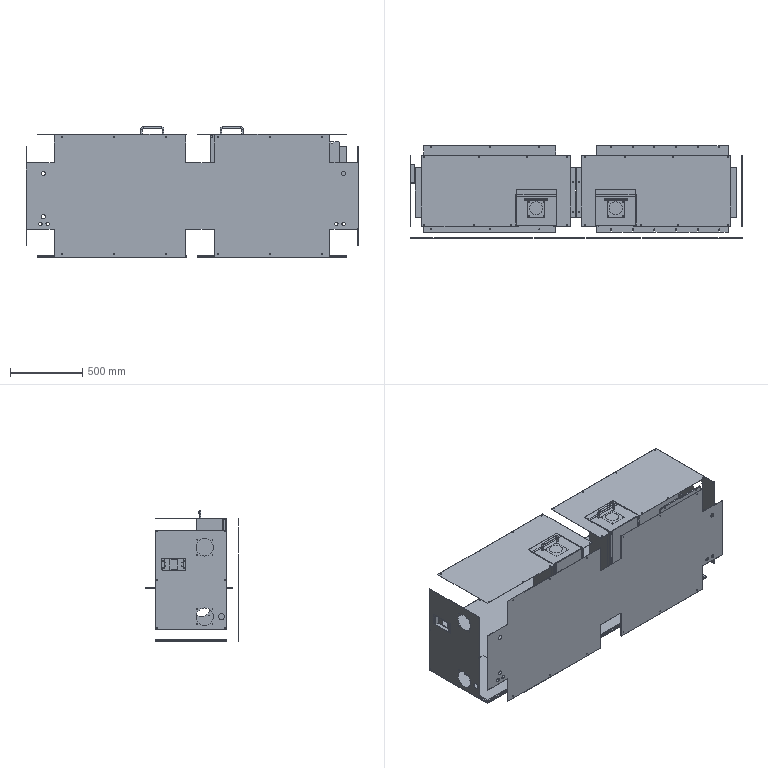Part | NX | 24 solids | 1005 faces | box 2300 x 642 x 903 mm | volume 15829508 mm3 | cylinder 466 | plane 377 | cone 94 | torus 56 | sphere 12 | commonest cylinder face diameters 7 x114 4 x80 5 x44 10 x32 12 x32 6.5 x24